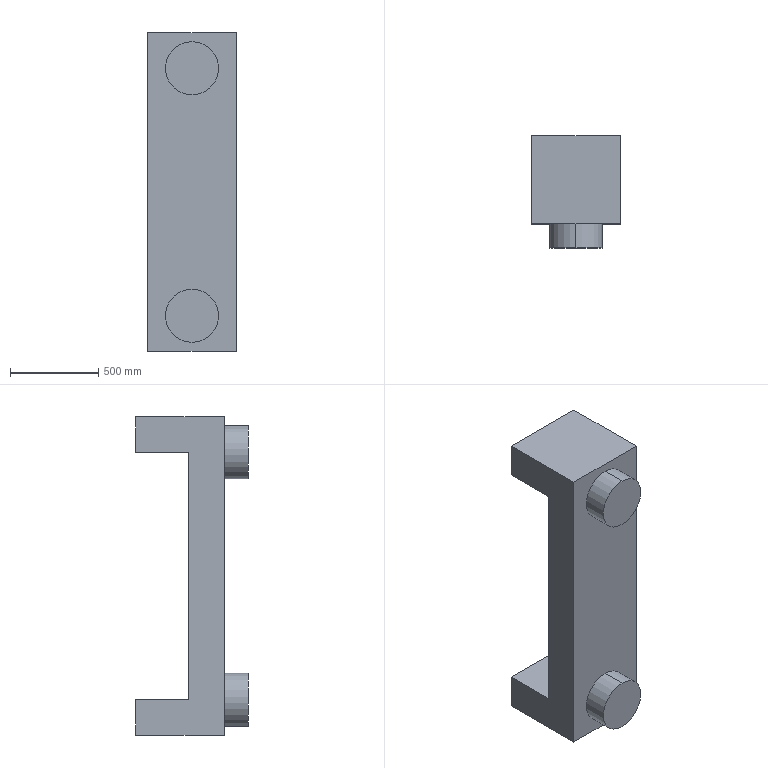Part | SolidWorks | features ICE 2, Extrusion 1 | 1 solid | 16 faces | box 500 x 636 x 1800 mm | volume 259226547 mm3 | plane 12 | cylinder 4 | commonest cylinder face diameters 300 x4
STEP:
#1=CARTESIAN_POINT('',(0.,-386.,550.));
#2=VERTEX_POINT('',#1);
#3=CARTESIAN_POINT('',(0.,-386.,850.));
#4=VERTEX_POINT('',#3);
#5=CARTESIAN_POINT('',(0.,-386.,700.));
#6=DIRECTION('',(0.,-1.,0.));
#7=DIRECTION('',(0.,0.,1.));
#8=AXIS2_PLACEMENT_3D('',#5,#6,#7);
#9=CIRCLE('',#8,150.);
#10=EDGE_CURVE('',#2,#4,#9,.T.);
#11=ORIENTED_EDGE('',*,*,#10,.F.);
#12=CARTESIAN_POINT('',(0.,-250.,550.));
#13=VERTEX_POINT('',#12);
#14=CARTESIAN_POINT('',(0.,-386.,550.));
#15=DIRECTION('',(0.,1.,0.));
#16=VECTOR('',#15,1000.);
#17=LINE('',#14,#16);
#18=EDGE_CURVE('',#2,#13,#17,.T.);
#19=ORIENTED_EDGE('',*,*,#18,.T.);
#20=CARTESIAN_POINT('',(0.,-250.,850.));
#21=VERTEX_POINT('',#20);
#22=CARTESIAN_POINT('',(0.,-250.,700.));
#23=DIRECTION('',(0.,-1.,0.));
#24=DIRECTION('',(0.,0.,1.));
#25=AXIS2_PLACEMENT_3D('',#22,#23,#24);
#26=CIRCLE('',#25,150.);
#27=EDGE_CURVE('',#13,#21,#26,.T.);
#28=ORIENTED_EDGE('',*,*,#27,.T.);
#29=CARTESIAN_POINT('',(0.,-386.,850.));
#30=DIRECTION('',(0.,1.,0.));
#31=VECTOR('',#30,1000.);
#32=LINE('',#29,#31);
#33=EDGE_CURVE('',#4,#21,#32,.T.);
#34=ORIENTED_EDGE('',*,*,#33,.F.);
#35=EDGE_LOOP('',(#11,#19,#28,#34));
#36=FACE_OUTER_BOUND('',#35,.T.);
#37=CARTESIAN_POINT('',(0.,-386.,700.));
#38=DIRECTION('',(0.,1.,0.));
#39=DIRECTION('',(0.,0.,1.));
#40=AXIS2_PLACEMENT_3D('',#37,#38,#39);
#41=CYLINDRICAL_SURFACE('',#40,150.);
#42=ADVANCED_FACE('',(#36),#41,.T.);
#43=CARTESIAN_POINT('',(0.,-386.,-850.));
#44=VERTEX_POINT('',#43);
#45=CARTESIAN_POINT('',(0.,-386.,-550.));
#46=VERTEX_POINT('',#45);
#47=CARTESIAN_POINT('',(0.,-386.,-700.));
#48=DIRECTION('',(0.,-1.,0.));
#49=DIRECTION('',(0.,0.,-1.));
#50=AXIS2_PLACEMENT_3D('',#47,#48,#49);
#51=CIRCLE('',#50,150.);
#52=EDGE_CURVE('',#44,#46,#51,.T.);
#53=ORIENTED_EDGE('',*,*,#52,.F.);
#54=CARTESIAN_POINT('',(0.,-250.,-850.));
#55=VERTEX_POINT('',#54);
#56=CARTESIAN_POINT('',(0.,-386.,-850.));
#57=DIRECTION('',(0.,1.,0.));
#58=VECTOR('',#57,1000.);
#59=LINE('',#56,#58);
#60=EDGE_CURVE('',#44,#55,#59,.T.);
#61=ORIENTED_EDGE('',*,*,#60,.T.);
#62=CARTESIAN_POINT('',(0.,-250.,-550.));
#63=VERTEX_POINT('',#62);
#64=CARTESIAN_POINT('',(0.,-250.,-700.));
#65=DIRECTION('',(0.,-1.,0.));
#66=DIRECTION('',(0.,0.,1.));
#67=AXIS2_PLACEMENT_3D('',#64,#65,#66);
#68=CIRCLE('',#67,150.);
#69=EDGE_CURVE('',#55,#63,#68,.T.);
#70=ORIENTED_EDGE('',*,*,#69,.T.);
#71=CARTESIAN_POINT('',(0.,-386.,-550.));
#72=DIRECTION('',(0.,1.,0.));
#73=VECTOR('',#72,1000.);
#74=LINE('',#71,#73);
#75=EDGE_CURVE('',#46,#63,#74,.T.);
#76=ORIENTED_EDGE('',*,*,#75,.F.);
#77=EDGE_LOOP('',(#53,#61,#70,#76));
#78=FACE_OUTER_BOUND('',#77,.T.);
#79=CARTESIAN_POINT('',(0.,-386.,-700.));
#80=DIRECTION('',(0.,1.,0.));
#81=DIRECTION('',(0.,0.,1.));
#82=AXIS2_PLACEMENT_3D('',#79,#80,#81);
#83=CYLINDRICAL_SURFACE('',#82,150.);
#84=ADVANCED_FACE('',(#78),#83,.T.);
#85=CARTESIAN_POINT('',(250.,250.,900.));
#86=VERTEX_POINT('',#85);
#87=CARTESIAN_POINT('',(250.,250.,700.));
#88=VERTEX_POINT('',#87);
#89=CARTESIAN_POINT('',(250.,250.,900.));
#90=DIRECTION('',(0.,0.,-1.));
#91=VECTOR('',#90,1000.);
#92=LINE('',#89,#91);
#93=EDGE_CURVE('',#86,#88,#92,.T.);
#94=ORIENTED_EDGE('',*,*,#93,.T.);
#95=CARTESIAN_POINT('',(-250.,250.,700.));
#96=VERTEX_POINT('',#95);
#97=CARTESIAN_POINT('',(-250.,250.,700.));
#98=DIRECTION('',(1.,0.,0.));
#99=VECTOR('',#98,1000.);
#100=LINE('',#97,#99);
#101=EDGE_CURVE('',#96,#88,#100,.T.);
#102=ORIENTED_EDGE('',*,*,#101,.F.);
#103=CARTESIAN_POINT('',(-250.,250.,900.));
#104=VERTEX_POINT('',#103);
#105=CARTESIAN_POINT('',(-250.,250.,900.));
#106=DIRECTION('',(0.,0.,-1.));
#107=VECTOR('',#106,1000.);
#108=LINE('',#105,#107);
#109=EDGE_CURVE('',#104,#96,#108,.T.);
#110=ORIENTED_EDGE('',*,*,#109,.F.);
#111=CARTESIAN_POINT('',(-250.,250.,900.));
#112=DIRECTION('',(-1.,0.,0.));
#113=VECTOR('',#112,1000.);
#114=LINE('',#111,#113);
#115=EDGE_CURVE('',#86,#104,#114,.T.);
#116=ORIENTED_EDGE('',*,*,#115,.F.);
#117=EDGE_LOOP('',(#94,#102,#110,#116));
#118=FACE_OUTER_BOUND('',#117,.T.);
#119=CARTESIAN_POINT('',(-250.,250.,900.));
#120=DIRECTION('',(0.,-1.,0.));
#121=DIRECTION('',(0.,0.,-1.));
#122=AXIS2_PLACEMENT_3D('',#119,#120,#121);
#123=PLANE('',#122);
#124=ADVANCED_FACE('',(#118),#123,.F.);
#125=CARTESIAN_POINT('',(250.,-50.,700.));
#126=VERTEX_POINT('',#125);
#127=CARTESIAN_POINT('',(250.,-50.,-700.));
#128=VERTEX_POINT('',#127);
#129=CARTESIAN_POINT('',(250.,-50.,700.));
#130=DIRECTION('',(0.,0.,-1.));
#131=VECTOR('',#130,1000.);
#132=LINE('',#129,#131);
#133=EDGE_CURVE('',#126,#128,#132,.T.);
#134=ORIENTED_EDGE('',*,*,#133,.F.);
#135=CARTESIAN_POINT('',(250.,250.,700.));
#136=DIRECTION('',(0.,-1.,0.));
#137=VECTOR('',#136,1000.);
#138=LINE('',#135,#137);
#139=EDGE_CURVE('',#88,#126,#138,.T.);
#140=ORIENTED_EDGE('',*,*,#139,.F.);
#141=ORIENTED_EDGE('',*,*,#93,.F.);
#142=CARTESIAN_POINT('',(250.,-250.,900.));
#143=VERTEX_POINT('',#142);
#144=CARTESIAN_POINT('',(250.,-250.,900.));
#145=DIRECTION('',(0.,1.,0.));
#146=VECTOR('',#145,1000.);
#147=LINE('',#144,#146);
#148=EDGE_CURVE('',#143,#86,#147,.T.);
#149=ORIENTED_EDGE('',*,*,#148,.F.);
#150=CARTESIAN_POINT('',(250.,-250.,-900.));
#151=VERTEX_POINT('',#150);
#152=CARTESIAN_POINT('',(250.,-250.,900.));
#153=DIRECTION('',(0.,0.,-1.));
#154=VECTOR('',#153,1000.);
#155=LINE('',#152,#154);
#156=EDGE_CURVE('',#143,#151,#155,.T.);
#157=ORIENTED_EDGE('',*,*,#156,.T.);
#158=CARTESIAN_POINT('',(250.,250.,-900.));
#159=VERTEX_POINT('',#158);
#160=CARTESIAN_POINT('',(250.,-250.,-900.));
#161=DIRECTION('',(0.,1.,0.));
#162=VECTOR('',#161,1000.);
#163=LINE('',#160,#162);
#164=EDGE_CURVE('',#151,#159,#163,.T.);
#165=ORIENTED_EDGE('',*,*,#164,.T.);
#166=CARTESIAN_POINT('',(250.,250.,-700.));
#167=VERTEX_POINT('',#166);
#168=CARTESIAN_POINT('',(250.,250.,900.));
#169=DIRECTION('',(0.,0.,-1.));
#170=VECTOR('',#169,1000.);
#171=LINE('',#168,#170);
#172=EDGE_CURVE('',#167,#159,#171,.T.);
#173=ORIENTED_EDGE('',*,*,#172,.F.);
#174=CARTESIAN_POINT('',(250.,250.,-700.));
#175=DIRECTION('',(0.,1.,0.));
#176=VECTOR('',#175,1000.);
#177=LINE('',#174,#176);
#178=EDGE_CURVE('',#128,#167,#177,.T.);
#179=ORIENTED_EDGE('',*,*,#178,.F.);
#180=EDGE_LOOP('',(#134,#140,#141,#149,#157,#165,#173,#179));
#181=FACE_OUTER_BOUND('',#180,.T.);
#182=CARTESIAN_POINT('',(250.,-250.,900.));
#183=DIRECTION('',(-1.,0.,0.));
#184=DIRECTION('',(0.,0.,1.));
#185=AXIS2_PLACEMENT_3D('',#182,#183,#184);
#186=PLANE('',#185);
#187=ADVANCED_FACE('',(#181),#186,.F.);
#188=CARTESIAN_POINT('',(-250.,250.,-700.));
#189=VERTEX_POINT('',#188);
#190=CARTESIAN_POINT('',(-250.,250.,-900.));
#191=VERTEX_POINT('',#190);
#192=CARTESIAN_POINT('',(-250.,250.,900.));
#193=DIRECTION('',(0.,0.,-1.));
#194=VECTOR('',#193,1000.);
#195=LINE('',#192,#194);
#196=EDGE_CURVE('',#189,#191,#195,.T.);
#197=ORIENTED_EDGE('',*,*,#196,.F.);
#198=CARTESIAN_POINT('',(-250.,250.,-700.));
#199=DIRECTION('',(1.,0.,0.));
#200=VECTOR('',#199,1000.);
#201=LINE('',#198,#200);
#202=EDGE_CURVE('',#189,#167,#201,.T.);
#203=ORIENTED_EDGE('',*,*,#202,.T.);
#204=ORIENTED_EDGE('',*,*,#172,.T.);
#205=CARTESIAN_POINT('',(-250.,250.,-900.));
#206=DIRECTION('',(-1.,0.,0.));
#207=VECTOR('',#206,1000.);
#208=LINE('',#205,#207);
#209=EDGE_CURVE('',#159,#191,#208,.T.);
#210=ORIENTED_EDGE('',*,*,#209,.T.);
#211=EDGE_LOOP('',(#197,#203,#204,#210));
#212=FACE_OUTER_BOUND('',#211,.T.);
#213=CARTESIAN_POINT('',(-250.,250.,900.));
#214=DIRECTION('',(0.,-1.,0.));
#215=DIRECTION('',(0.,0.,-1.));
#216=AXIS2_PLACEMENT_3D('',#213,#214,#215);
#217=PLANE('',#216);
#218=ADVANCED_FACE('',(#212),#217,.F.);
#219=ORIENTED_EDGE('',*,*,#109,.T.);
#220=CARTESIAN_POINT('',(-250.,-50.,700.));
#221=VERTEX_POINT('',#220);
#222=CARTESIAN_POINT('',(-250.,250.,700.));
#223=DIRECTION('',(0.,-1.,0.));
#224=VECTOR('',#223,1000.);
#225=LINE('',#222,#224);
#226=EDGE_CURVE('',#96,#221,#225,.T.);
#227=ORIENTED_EDGE('',*,*,#226,.T.);
#228=CARTESIAN_POINT('',(-250.,-50.,-700.));
#229=VERTEX_POINT('',#228);
#230=CARTESIAN_POINT('',(-250.,-50.,700.));
#231=DIRECTION('',(0.,0.,-1.));
#232=VECTOR('',#231,1000.);
#233=LINE('',#230,#232);
#234=EDGE_CURVE('',#221,#229,#233,.T.);
#235=ORIENTED_EDGE('',*,*,#234,.T.);
#236=CARTESIAN_POINT('',(-250.,250.,-700.));
#237=DIRECTION('',(0.,1.,0.));
#238=VECTOR('',#237,1000.);
#239=LINE('',#236,#238);
#240=EDGE_CURVE('',#229,#189,#239,.T.);
#241=ORIENTED_EDGE('',*,*,#240,.T.);
#242=ORIENTED_EDGE('',*,*,#196,.T.);
#243=CARTESIAN_POINT('',(-250.,-250.,-900.));
#244=VERTEX_POINT('',#243);
#245=CARTESIAN_POINT('',(-250.,-250.,-900.));
#246=DIRECTION('',(0.,-1.,0.));
#247=VECTOR('',#246,1000.);
#248=LINE('',#245,#247);
#249=EDGE_CURVE('',#191,#244,#248,.T.);
#250=ORIENTED_EDGE('',*,*,#249,.T.);
#251=CARTESIAN_POINT('',(-250.,-250.,900.));
#252=VERTEX_POINT('',#251);
#253=CARTESIAN_POINT('',(-250.,-250.,900.));
#254=DIRECTION('',(0.,0.,-1.));
#255=VECTOR('',#254,1000.);
#256=LINE('',#253,#255);
#257=EDGE_CURVE('',#252,#244,#256,.T.);
#258=ORIENTED_EDGE('',*,*,#257,.F.);
#259=CARTESIAN_POINT('',(-250.,-250.,900.));
#260=DIRECTION('',(0.,-1.,0.));
#261=VECTOR('',#260,1000.);
#262=LINE('',#259,#261);
#263=EDGE_CURVE('',#104,#252,#262,.T.);
#264=ORIENTED_EDGE('',*,*,#263,.F.);
#265=EDGE_LOOP('',(#219,#227,#235,#241,#242,#250,#258,#264));
#266=FACE_OUTER_BOUND('',#265,.T.);
#267=CARTESIAN_POINT('',(-250.,-250.,900.));
#268=DIRECTION('',(1.,0.,0.));
#269=DIRECTION('',(0.,0.,-1.));
#270=AXIS2_PLACEMENT_3D('',#267,#268,#269);
#271=PLANE('',#270);
#272=ADVANCED_FACE('',(#266),#271,.F.);
#273=CARTESIAN_POINT('',(0.,-250.,700.));
#274=DIRECTION('',(0.,-1.,0.));
#275=DIRECTION('',(0.,0.,1.));
#276=AXIS2_PLACEMENT_3D('',#273,#274,#275);
#277=CIRCLE('',#276,150.);
#278=EDGE_CURVE('',#21,#13,#277,.T.);
#279=ORIENTED_EDGE('',*,*,#278,.F.);
#280=ORIENTED_EDGE('',*,*,#27,.F.);
#281=EDGE_LOOP('',(#279,#280));
#282=FACE_BOUND('',#281,.T.);
#283=CARTESIAN_POINT('',(0.,-250.,-700.));
#284=DIRECTION('',(0.,-1.,0.));
#285=DIRECTION('',(0.,0.,1.));
#286=AXIS2_PLACEMENT_3D('',#283,#284,#285);
#287=CIRCLE('',#286,150.);
#288=EDGE_CURVE('',#63,#55,#287,.T.);
#289=ORIENTED_EDGE('',*,*,#288,.F.);
#290=ORIENTED_EDGE('',*,*,#69,.F.);
#291=EDGE_LOOP('',(#289,#290));
#292=FACE_BOUND('',#291,.T.);
#293=CARTESIAN_POINT('',(-250.,-250.,-900.));
#294=DIRECTION('',(1.,0.,0.));
#295=VECTOR('',#294,1000.);
#296=LINE('',#293,#295);
#297=EDGE_CURVE('',#244,#151,#296,.T.);
#298=ORIENTED_EDGE('',*,*,#297,.T.);
#299=ORIENTED_EDGE('',*,*,#156,.F.);
#300=CARTESIAN_POINT('',(-250.,-250.,900.));
#301=DIRECTION('',(1.,0.,0.));
#302=VECTOR('',#301,1000.);
#303=LINE('',#300,#302);
#304=EDGE_CURVE('',#252,#143,#303,.T.);
#305=ORIENTED_EDGE('',*,*,#304,.F.);
#306=ORIENTED_EDGE('',*,*,#257,.T.);
#307=EDGE_LOOP('',(#298,#299,#305,#306));
#308=FACE_OUTER_BOUND('',#307,.T.);
#309=CARTESIAN_POINT('',(-250.,-250.,900.));
#310=DIRECTION('',(0.,1.,0.));
#311=DIRECTION('',(0.,0.,1.));
#312=AXIS2_PLACEMENT_3D('',#309,#310,#311);
#313=PLANE('',#312);
#314=ADVANCED_FACE('',(#282,#292,#308),#313,.F.);
#315=ORIENTED_EDGE('',*,*,#148,.T.);
#316=ORIENTED_EDGE('',*,*,#115,.T.);
#317=ORIENTED_EDGE('',*,*,#263,.T.);
#318=ORIENTED_EDGE('',*,*,#304,.T.);
#319=EDGE_LOOP('',(#315,#316,#317,#318));
#320=FACE_OUTER_BOUND('',#319,.T.);
#321=CARTESIAN_POINT('',(0.,0.,900.));
#322=DIRECTION('',(0.,0.,-1.));
#323=DIRECTION('',(-1.,0.,0.));
#324=AXIS2_PLACEMENT_3D('',#321,#322,#323);
#325=PLANE('',#324);
#326=ADVANCED_FACE('',(#320),#325,.F.);
#327=ORIENTED_EDGE('',*,*,#164,.F.);
#328=ORIENTED_EDGE('',*,*,#297,.F.);
#329=ORIENTED_EDGE('',*,*,#249,.F.);
#330=ORIENTED_EDGE('',*,*,#209,.F.);
#331=EDGE_LOOP('',(#327,#328,#329,#330));
#332=FACE_OUTER_BOUND('',#331,.T.);
#333=CARTESIAN_POINT('',(0.,0.,-900.));
#334=DIRECTION('',(0.,0.,-1.));
#335=DIRECTION('',(-1.,0.,0.));
#336=AXIS2_PLACEMENT_3D('',#333,#334,#335);
#337=PLANE('',#336);
#338=ADVANCED_FACE('',(#332),#337,.T.);
#339=ORIENTED_EDGE('',*,*,#60,.F.);
#340=CARTESIAN_POINT('',(0.,-386.,-700.));
#341=DIRECTION('',(0.,-1.,0.));
#342=DIRECTION('',(0.,0.,-1.));
#343=AXIS2_PLACEMENT_3D('',#340,#341,#342);
#344=CIRCLE('',#343,150.);
#345=EDGE_CURVE('',#46,#44,#344,.T.);
#346=ORIENTED_EDGE('',*,*,#345,.F.);
#347=ORIENTED_EDGE('',*,*,#75,.T.);
#348=ORIENTED_EDGE('',*,*,#288,.T.);
#349=EDGE_LOOP('',(#339,#346,#347,#348));
#350=FACE_OUTER_BOUND('',#349,.T.);
#351=CARTESIAN_POINT('',(0.,-386.,-700.));
#352=DIRECTION('',(0.,1.,0.));
#353=DIRECTION('',(0.,0.,1.));
#354=AXIS2_PLACEMENT_3D('',#351,#352,#353);
#355=CYLINDRICAL_SURFACE('',#354,150.);
#356=ADVANCED_FACE('',(#350),#355,.T.);
#357=ORIENTED_EDGE('',*,*,#345,.T.);
#358=ORIENTED_EDGE('',*,*,#52,.T.);
#359=EDGE_LOOP('',(#357,#358));
#360=FACE_OUTER_BOUND('',#359,.T.);
#361=CARTESIAN_POINT('',(0.,-386.,-700.));
#362=DIRECTION('',(0.,-1.,0.));
#363=DIRECTION('',(0.,0.,-1.));
#364=AXIS2_PLACEMENT_3D('',#361,#362,#363);
#365=PLANE('',#364);
#366=ADVANCED_FACE('',(#360),#365,.T.);
#367=ORIENTED_EDGE('',*,*,#18,.F.);
#368=CARTESIAN_POINT('',(0.,-386.,700.));
#369=DIRECTION('',(0.,-1.,0.));
#370=DIRECTION('',(0.,0.,1.));
#371=AXIS2_PLACEMENT_3D('',#368,#369,#370);
#372=CIRCLE('',#371,150.);
#373=EDGE_CURVE('',#4,#2,#372,.T.);
#374=ORIENTED_EDGE('',*,*,#373,.F.);
#375=ORIENTED_EDGE('',*,*,#33,.T.);
#376=ORIENTED_EDGE('',*,*,#278,.T.);
#377=EDGE_LOOP('',(#367,#374,#375,#376));
#378=FACE_OUTER_BOUND('',#377,.T.);
#379=CARTESIAN_POINT('',(0.,-386.,700.));
#380=DIRECTION('',(0.,1.,0.));
#381=DIRECTION('',(0.,0.,1.));
#382=AXIS2_PLACEMENT_3D('',#379,#380,#381);
#383=CYLINDRICAL_SURFACE('',#382,150.);
#384=ADVANCED_FACE('',(#378),#383,.T.);
#385=ORIENTED_EDGE('',*,*,#373,.T.);
#386=ORIENTED_EDGE('',*,*,#10,.T.);
#387=EDGE_LOOP('',(#385,#386));
#388=FACE_OUTER_BOUND('',#387,.T.);
#389=CARTESIAN_POINT('',(0.,-386.,700.));
#390=DIRECTION('',(0.,1.,0.));
#391=DIRECTION('',(0.,0.,1.));
#392=AXIS2_PLACEMENT_3D('',#389,#390,#391);
#393=PLANE('',#392);
#394=ADVANCED_FACE('',(#388),#393,.F.);
#395=ORIENTED_EDGE('',*,*,#139,.T.);
#396=CARTESIAN_POINT('',(-250.,-50.,700.));
#397=DIRECTION('',(1.,0.,0.));
#398=VECTOR('',#397,1000.);
#399=LINE('',#396,#398);
#400=EDGE_CURVE('',#221,#126,#399,.T.);
#401=ORIENTED_EDGE('',*,*,#400,.F.);
#402=ORIENTED_EDGE('',*,*,#226,.F.);
#403=ORIENTED_EDGE('',*,*,#101,.T.);
#404=EDGE_LOOP('',(#395,#401,#402,#403));
#405=FACE_OUTER_BOUND('',#404,.T.);
#406=CARTESIAN_POINT('',(-250.,250.,700.));
#407=DIRECTION('',(0.,0.,1.));
#408=DIRECTION('',(1.,0.,0.));
#409=AXIS2_PLACEMENT_3D('',#406,#407,#408);
#410=PLANE('',#409);
#411=ADVANCED_FACE('',(#405),#410,.F.);
#412=ORIENTED_EDGE('',*,*,#178,.T.);
#413=ORIENTED_EDGE('',*,*,#202,.F.);
#414=ORIENTED_EDGE('',*,*,#240,.F.);
#415=CARTESIAN_POINT('',(-250.,-50.,-700.));
#416=DIRECTION('',(1.,0.,0.));
#417=VECTOR('',#416,1000.);
#418=LINE('',#415,#417);
#419=EDGE_CURVE('',#229,#128,#418,.T.);
#420=ORIENTED_EDGE('',*,*,#419,.T.);
#421=EDGE_LOOP('',(#412,#413,#414,#420));
#422=FACE_OUTER_BOUND('',#421,.T.);
#423=CARTESIAN_POINT('',(-250.,250.,-700.));
#424=DIRECTION('',(0.,0.,-1.));
#425=DIRECTION('',(-1.,0.,0.));
#426=AXIS2_PLACEMENT_3D('',#423,#424,#425);
#427=PLANE('',#426);
#428=ADVANCED_FACE('',(#422),#427,.F.);
#429=ORIENTED_EDGE('',*,*,#133,.T.);
#430=ORIENTED_EDGE('',*,*,#419,.F.);
#431=ORIENTED_EDGE('',*,*,#234,.F.);
#432=ORIENTED_EDGE('',*,*,#400,.T.);
#433=EDGE_LOOP('',(#429,#430,#431,#432));
#434=FACE_OUTER_BOUND('',#433,.T.);
#435=CARTESIAN_POINT('',(-250.,-50.,700.));
#436=DIRECTION('',(0.,-1.,0.));
#437=DIRECTION('',(0.,0.,-1.));
#438=AXIS2_PLACEMENT_3D('',#435,#436,#437);
#439=PLANE('',#438);
#440=ADVANCED_FACE('',(#434),#439,.F.);
#441=CLOSED_SHELL('',(#42,#84,#124,#187,#218,#272,#314,#326,#338,#356,#366,#384,#394,#411,#428,#440));
#442=MANIFOLD_SOLID_BREP('',#441);
#443=CARTESIAN_POINT('',(0.,0.,0.));
#444=DIRECTION('',(0.,0.,1.));
#445=DIRECTION('',(1.,0.,0.));
#446=AXIS2_PLACEMENT_3D('',#443,#444,#445);
#447=(LENGTH_UNIT()NAMED_UNIT(*)SI_UNIT(.MILLI.,.METRE.));
#448=UNCERTAINTY_MEASURE_WITH_UNIT(LENGTH_MEASURE(0.00001),#447,'','');
#449=(NAMED_UNIT(*)PLANE_ANGLE_UNIT()SI_UNIT($,.RADIAN.));
#450=(NAMED_UNIT(*)SI_UNIT($,.STERADIAN.)SOLID_ANGLE_UNIT());
#451=(GEOMETRIC_REPRESENTATION_CONTEXT(3)GLOBAL_UNCERTAINTY_ASSIGNED_CONTEXT((#448))GLOBAL_UNIT_ASSIGNED_CONTEXT((#447,#449,#450))REPRESENTATION_CONTEXT('',''));
#452=ADVANCED_BREP_SHAPE_REPRESENTATION('',(#442,#446),#451);